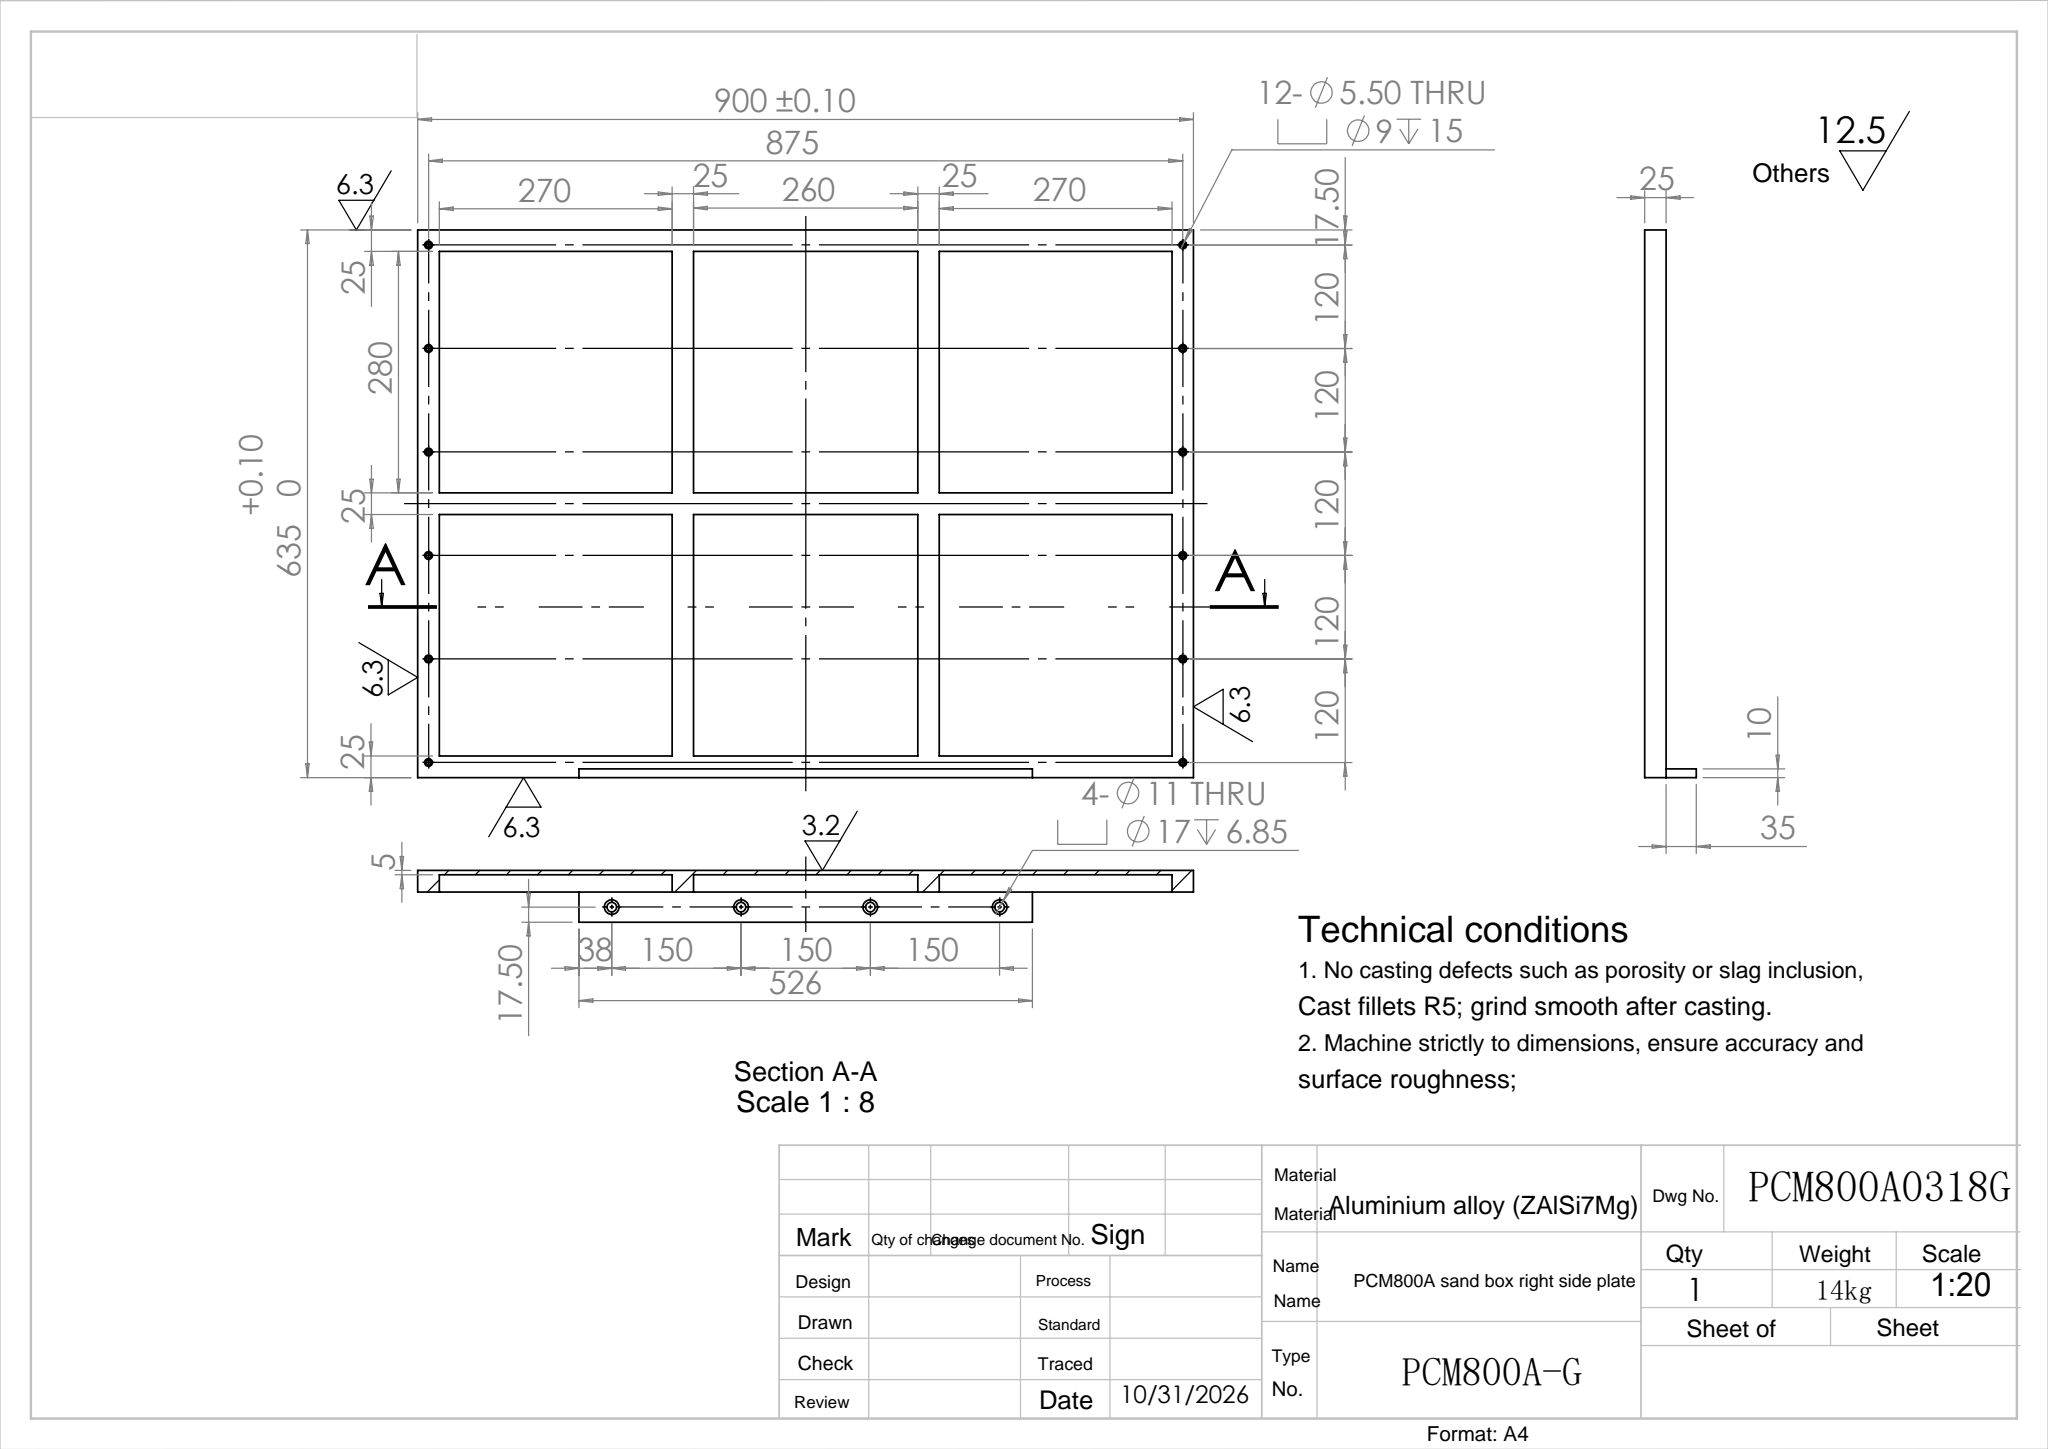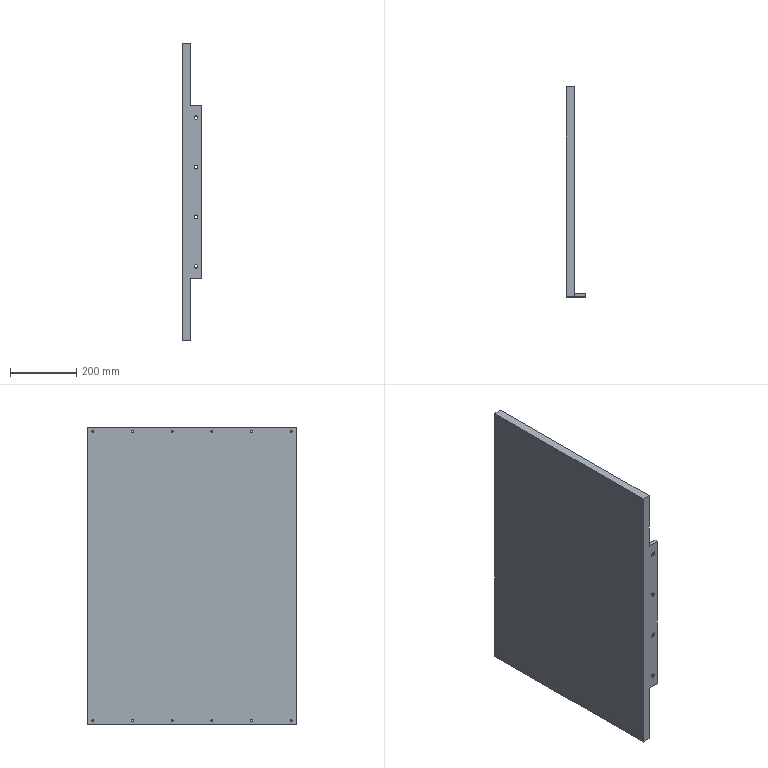Part | SolidWorks | features Boss 5, 3DProfileFeature 2, HoleWzd 2, Extrusion 1, MirrorPattern 1 | 1 solid | 120 faces | box 60 x 635 x 900 mm | volume 5489881 mm3 | cylinder 64 | plane 56 | commonest cylinder face diameters 5.5 x24 9 x24 11 x8 17 x8